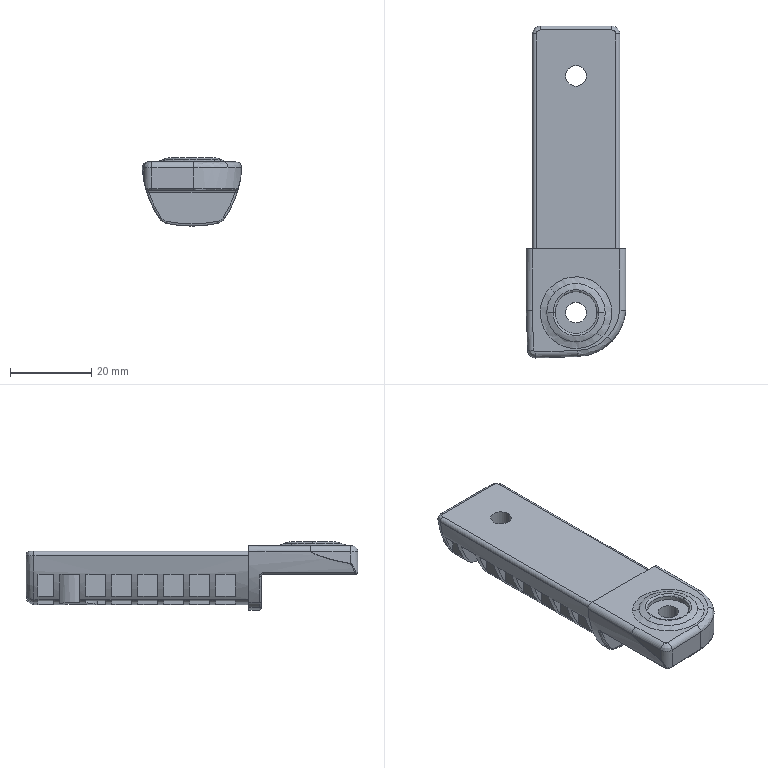Part | SolidWorks | features BaseBody 1 | 1 solid | 242 faces | box 24.436 x 81.569 x 16.763 mm | volume 14463 mm3 | plane 145 | cylinder 63 | spline 34 | commonest cylinder face diameters 3.137 x18 0.98 x15 10.98 x5 2.941 x4 5.098 x4 1.961 x3